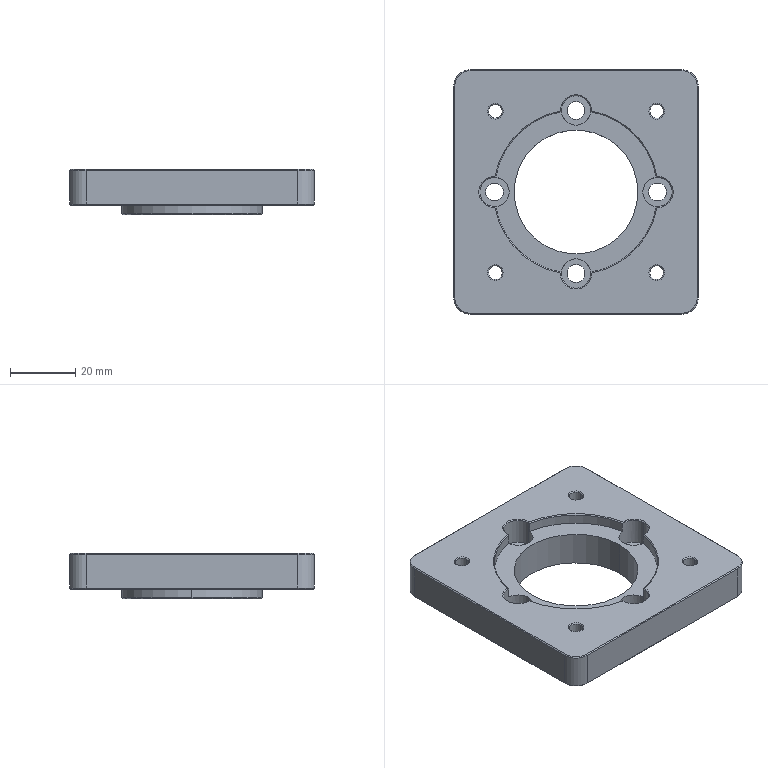Part | STEP file | 1 solid | 86 faces | box 75 x 75 x 14 mm | volume 44712 mm3 | cylinder 36 | cone 30 | plane 20 | commonest cylinder face diameters 4.2 x8 5.5 x8 9 x8 10 x4 50.1 x4 38 x2